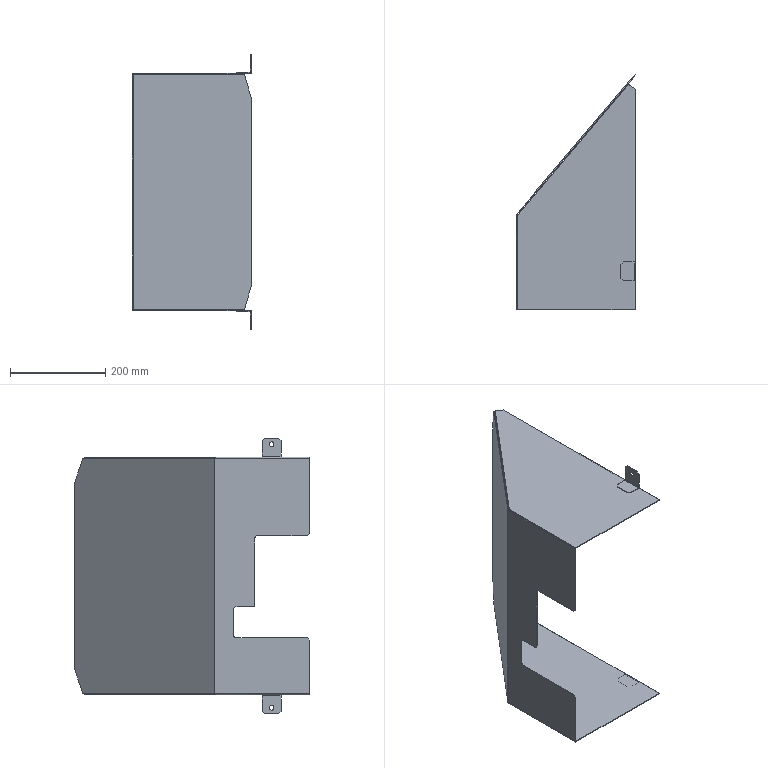Part | SolidWorks | features FlatPattern 3, BreakCorner 2, ICE 2, SheetMetal 2, EdgeFlange 1, Extrusion 1, Fillet 1, HoleWzd 1, MirrorSolid 1, SMBaseFlange 1, SolidToSheetMetal 1 | 3 solids | 89 faces | box 251.144 x 495 x 580 mm | volume 655996 mm3 | plane 66 | cylinder 18 | spline 5 | commonest cylinder face diameters 10 x8 1.473 x5 4.473 x5